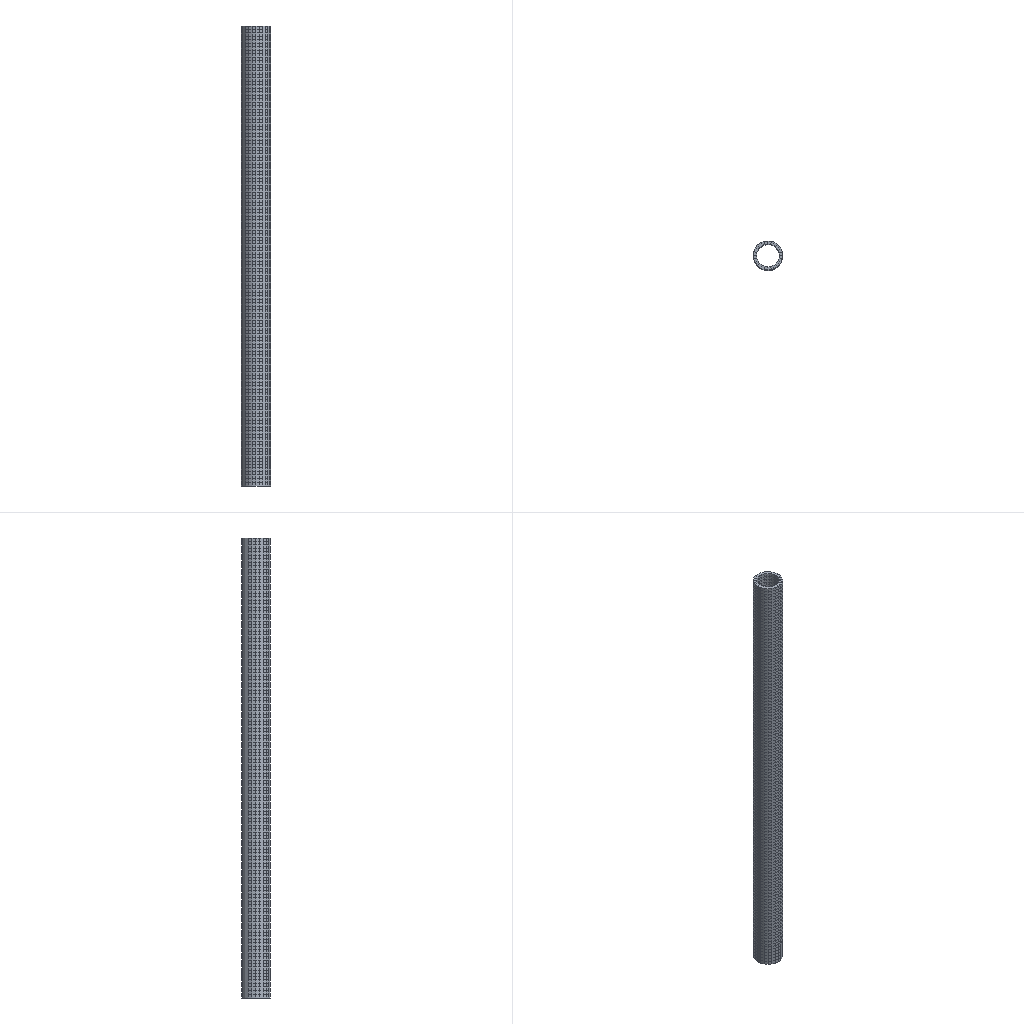Simulation study | abaqus
Set-up summary:
category,name,step,type,value,unit,region
solver,abaqus,,Abaqus/CAE 2024
units,mm-N-s-tonne (MPa),,inferred,E=210000 density=
analysis,Step-4,,static,time_period=10
mesh,nodes,,,6969
mesh,elements,,,3458
element_type,C3D8R,,,3458
material,Material-1,,E,210000
material,Material-1,,nu,0.3
material,Material-1,,yield,380
material,Material-1,,cte,1.3e-05
material,Material-1,,behaviors,plastic; expansion
section,Material-1,,solid section,,,Set-1
load,Load-2,Step-4,pressure,30,,Surf-6
load,Load-4,Step-4,concentrated force,"1000 [dir=(0, 1, 0)]",,Set-13
bc,BC-1,initial,fixed,"[dofs=rx,ry,rz,x,y,z n=6]",,Set-5
bc,BC-2,Step-4,displacement,-0.5 [dofs=rx],,_PickedSet34
bc,BC-2,Step-4,fixed,"[dofs=ry,rz n=2]",,_PickedSet34
constraint,coupling,,,1
Abaqus input file, long lists of numbers shortened:
*Heading
** Job name: deck Model name: Model-1-1
** Generated by: Abaqus/CAE 2024
*Preprint, echo=NO, model=NO, history=NO, contact=NO
**
** PARTS
**
*Part, name=Part-10
*Node
      1,           0.,          62.,         120.
      2,           0.,          50.,         120.
** (6966 more lines like these left out)
*Element, type=C3D8R
   1,    1,    2,   33,    5,   56,  303,  989,  551
   2,    5,   33,   34,   49,  551,  989,  990, 2612
** (3456 more lines like these left out)
*Nset, nset=Set-1, generate
    1,  6968,     1
*Elset, elset=Set-1, generate
    1,  3458,     1
** Section: Section-1
*Solid Section, elset=Set-1, material=Material-1
,
*End Part
**
**
** ASSEMBLY
**
*Assembly, name=Assembly
**
*Instance, name=Part-10-1, part=Part-10
*End Instance
**
*Node
      1,           0., -3.91886993e-15,        2000.
*Nset, nset=Set-5, instance=Part-10-1
  22,  23,  24,  25,  26,  30,  31,  32, 916, 917, 918, 919, 920, 921, 922, 923
 924, 925, 926, 927, 928, 929, 930, 931, 932, 933, 934, 935, 936, 966, 967, 968
** (2 more lines like these left out)
*Elset, elset=Set-5, instance=Part-10-1
 3335, 3336, 3337, 3338, 3339, 3340, 3341, 3342, 3343, 3344, 3345, 3346, 3445, 3446, 3447, 3448
 3449, 3450, 3451, 3452, 3453, 3454, 3455, 3456, 3457, 3458
*Nset, nset=Set-13
 1,
*Nset, nset=m_Set-12
 1,
*Nset, nset=s_Set-8, instance=Part-10-1
   8,   9,  10,  11,  12,  13,  14,  16, 676, 677, 678, 679, 680, 681, 682, 683
 684, 685, 686, 687, 688, 689, 690, 691, 692, 693, 694, 695, 696, 697, 698, 844
** (2 more lines like these left out)
*Elset, elset=s_Set-8, instance=Part-10-1
 1737, 1738, 1739, 1740, 1741, 1742, 1743, 1744, 1745, 1746, 1747, 1748, 1749, 1750, 3239, 3240
 3241, 3242, 3243, 3244, 3245, 3246, 3247, 3248, 3249, 3250
*Nset, nset=_PickedSet34, internal
 1,
*Elset, elset=_Surf-2_S3, internal, instance=Part-10-1, generate
 3251,  3346,     1
*Elset, elset=_Surf-2_S5, internal, instance=Part-10-1, generate
 3347,  3458,     1
*Elset, elset=_Surf-2_S4, internal, instance=Part-10-1, generate
    1,  1750,     1
*Elset, elset=_Surf-2_S6, internal, instance=Part-10-1, generate
 1751,  3250,     1
*Surface, type=ELEMENT, name=Surf-2
_Surf-2_S3, S3
_Surf-2_S5, S5
_Surf-2_S4, S4
_Surf-2_S6, S6
*Elset, elset=_Surf-5_S5, internal, instance=Part-10-1
 3288, 3289, 3290, 3291, 3292, 3293, 3294, 3295, 3296, 3297, 3298, 3300, 3301, 3302, 3303, 3304
 3305, 3306, 3307, 3308, 3309, 3310, 3312, 3313, 3314, 3315, 3316, 3317, 3318, 3319, 3320, 3321
** (2 more lines like these left out)
*Elset, elset=_Surf-5_S3, internal, instance=Part-10-1
 3390, 3391, 3392, 3393, 3394, 3395, 3396, 3397, 3398, 3399, 3400, 3401, 3402, 3404, 3405, 3406
 3407, 3408, 3409, 3410, 3411, 3412, 3413, 3414, 3415, 3416, 3418, 3419, 3420, 3421, 3422, 3423
** (3 more lines like these left out)
*Elset, elset=_Surf-5_S4, internal, instance=Part-10-1
 1752, 1753, 1754, 1755, 1756, 1757, 1758, 1759, 1760, 1761, 1762, 1764, 1765, 1766, 1767, 1768
 1769, 1770, 1771, 1772, 1773, 1774, 1776, 1777, 1778, 1779, 1780, 1781, 1782, 1783, 1784, 1785
** (84 more lines like these left out)
*Elset, elset=_Surf-5_S6, internal, instance=Part-10-1
    2,    3,    4,    5,    6,    7,    8,    9,   10,   11,   12,   13,   14,   16,   17,   18
   19,   20,   21,   22,   23,   24,   25,   26,   27,   28,   30,   31,   32,   33,   34,   35
** (100 more lines like these left out)
*Surface, type=ELEMENT, name=Surf-5
_Surf-5_S5, S5
_Surf-5_S3, S3
_Surf-5_S4, S4
_Surf-5_S6, S6
*Elset, elset=_Surf-6_S3, internal, instance=Part-10-1, generate
 3347,  3458,     1
*Elset, elset=_Surf-6_S5, internal, instance=Part-10-1, generate
 3251,  3346,     1
*Elset, elset=_Surf-6_S4, internal, instance=Part-10-1, generate
 1751,  3250,     1
*Elset, elset=_Surf-6_S6, internal, instance=Part-10-1, generate
    1,  1750,     1
*Surface, type=ELEMENT, name=Surf-6
_Surf-6_S3, S3
_Surf-6_S5, S5
_Surf-6_S4, S4
_Surf-6_S6, S6
*Elset, elset=_m_Surf-3_S2, internal, instance=Part-10-1
 1737, 1738, 1739, 1740, 1741, 1742, 1743, 1744, 1745, 1746, 1747, 1748, 1749, 1750, 3239, 3240
 3241, 3242, 3243, 3244, 3245, 3246, 3247, 3248, 3249, 3250
*Surface, type=ELEMENT, name=m_Surf-3
_m_Surf-3_S2, S2
*Elset, elset=_s_Surf-4_S2, internal, instance=Part-10-1
 1737, 1738, 1739, 1740, 1741, 1742, 1743, 1744, 1745, 1746, 1747, 1748, 1749, 1750, 3239, 3240
 3241, 3242, 3243, 3244, 3245, 3246, 3247, 3248, 3249, 3250
*Surface, type=ELEMENT, name=s_Surf-4
_s_Surf-4_S2, S2
** Constraint: Constraint-3
*Coupling, constraint name=Constraint-3, ref node=m_Set-12, surface=s_Surf-4
*Kinematic
*End Assembly
**
** MATERIALS
**
*Material, name=Material-1
*Elastic
210000., 0.3
*Expansion
 1.3e-05,
*Plastic
380.,  0.
600., 0.2
**
** BOUNDARY CONDITIONS
**
** Name: BC-1 Type: Displacement/Rotation
*Boundary
Set-5, 1, 1
Set-5, 2, 2
Set-5, 3, 3
Set-5, 4, 4
Set-5, 5, 5
Set-5, 6, 6
** ----------------------------------------------------------------
**
** STEP: Step-4
**
*Step, name=Step-4, nlgeom=NO, inc=1000
*Static
1., 10., 0.0001, 1.
**
** BOUNDARY CONDITIONS
**
** Name: BC-2 Type: Displacement/Rotation
*Boundary
_PickedSet34, 4, 4, -0.5
_PickedSet34, 5, 5
_PickedSet34, 6, 6
**
** LOADS
**
** Name: Load-2   Type: Pressure
*Dsload
Surf-6, P, 30.
** Name: Load-4   Type: Concentrated force
*Cload
Set-13, 2, 1000.
**
** OUTPUT REQUESTS
**
*Restart, write, frequency=0
**
** FIELD OUTPUT: F-Output-2
**
*Output, field
*Node Output
CF, RF, RM, RT, TF, U, UR, UT
V, VF, VR, VT
*Element Output, directions=YES
ALPHA, ALPHAN, BF, CENTMAG, CENTRIFMAG, CORIOMAG, CS11, CTSHR, E, EE, EEQUT, ER, ESF1, GRAV, HP, IE
LE, LODE, MISES, MISESMAX, MISESONLY, NE, NFORC, NFORCSO, P, PE, PEEQ, PEEQMAX, PEEQT, PEMAG, PEQC, PRESSONLY
PS, ROTAMAG, S, SALPHA, SE, SEE, SEP, SEPE, SEQUT, SF, SPE, SQEQ, SSAVG, TE, TEEQ, TEVOL
THE, TRIAX, TRNOR, TRSHR, TSHR, VE, VEEQ, VS, YIELDPOT
**
** HISTORY OUTPUT: H-Output-2
**
*Output, history
*Element Output
IRA1, IRA2, IRA3, IRAR1, IRAR2, IRAR3, IRF1, IRF2, IRF3, IRM1, IRM2, IRM3
*End Step
Results summary:
result,odb.job_status,,,JOB_STATUS_COMPLETED_SUCCESSFULLY,"consistent, unstated (Abaqus has no unit system)"
result,steps[0].procedure,Step-4,,*STATIC,"consistent, unstated (Abaqus has no unit system)"
result,steps[0].time_period,Step-4,,10,"consistent, unstated (Abaqus has no unit system)"
result,steps[0].n_frames,Step-4,,14,"consistent, unstated (Abaqus has no unit system)"
result,steps[0].last_frame.id,Step-4,,13,"consistent, unstated (Abaqus has no unit system)"
result,steps[0].last_frame.value,Step-4,,10,"consistent, unstated (Abaqus has no unit system)"
result,steps[0].last_frame.description,Step-4,,Increment     13: Step Time =    10.00,"consistent, unstated (Abaqus has no unit system)"
result,steps[0].completed,Step-4,,True,"consistent, unstated (Abaqus has no unit system)"
result,steps[0].max_U_magnitude,Step-4,,551.846,"consistent, unstated (Abaqus has no unit system)"
result,steps[0].max_S_mises,Step-4,,407.752,"consistent, unstated (Abaqus has no unit system)"
result,steps[0].RF_sum[1],Step-4,,0.0005188,"consistent, unstated (Abaqus has no unit system)"
result,steps[0].RF_sum[2],Step-4,,-1000,"consistent, unstated (Abaqus has no unit system)"
result,steps[0].RF_sum[3],Step-4,,-0.007812,"consistent, unstated (Abaqus has no unit system)"